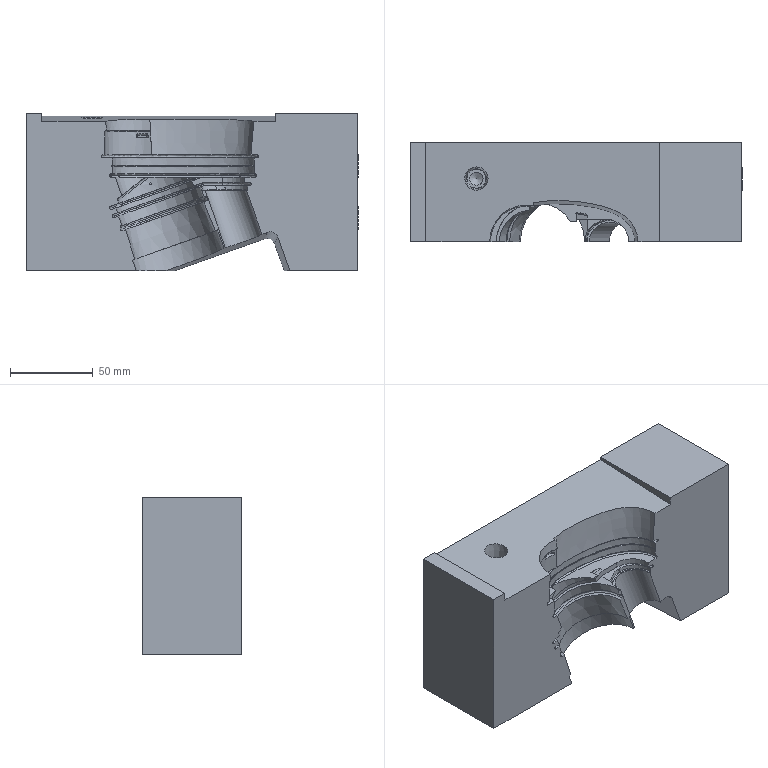Part | STEP file | CAV_id650_x_t | 1 solid | 116 faces | box 200 x 60 x 95 mm | volume 908524 mm3 | plane 43 | cylinder 32 | other 23 | cone 11 | spline 7 | commonest cylinder face diameters 1.934 x5 8 x5 2.036 x4 1.018 x3 59.553 x2 10 x1